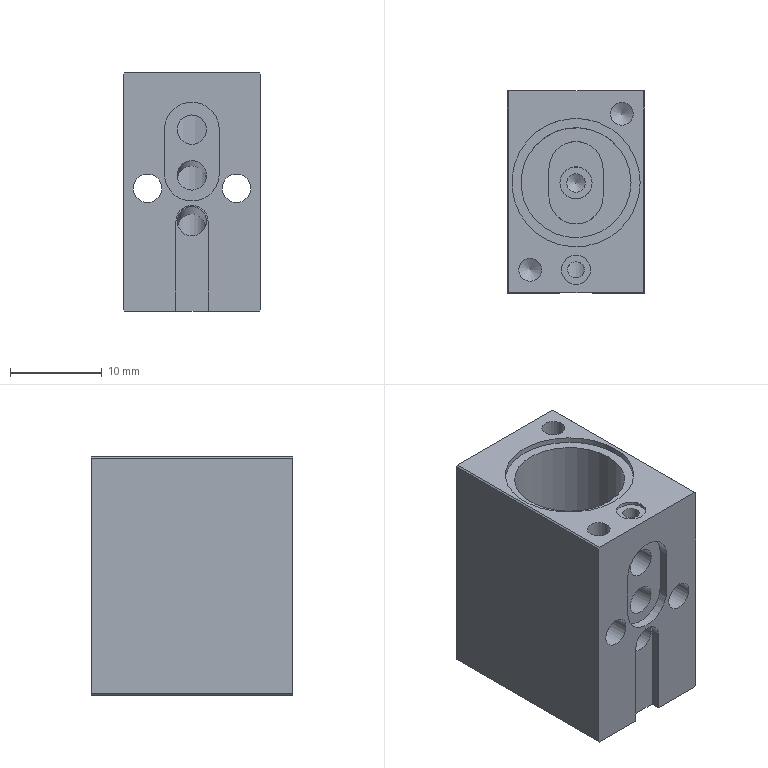NC program | NX | posted with a generic post | part box 15 x 22 x 26 mm
Whole program:
N10 G17 G21 G94 G90
(PLANAR_MILL_2_COPY , TOOL : D3精光)
N12 T05 M6
N14 G54
N16 G17 G0 G90 X-0.215 Y6.8 B0. C0. S3000 M3
N18 G43 Z30. H5
N20 Z1.02
N22 G94 G1 Z-0.98 F300.
N24 Y5.3
N26 G3 X1.285 Y6.8 R1.5
N28 X-0.015 Y8.1 R1.3
N30 X-1.315 Y6.8 R1.3
N32 G1 Y2.
N34 G3 X-0.015 Y0.7 R1.3
N36 X1.285 Y2. R1.3
N38 G1 Y6.8
N40 G3 X0.535 Y7.55 R0.75
N42 G1 Y6.8
N44 Z1.02
N46 G0 Z30.
(PLANAR_MILL_2_COPY_COPY , TOOL : D3精光)
N48 X-0.015
N50 Z1.02
N52 G1 Z-0.98
N54 Y5.3
N56 G3 X1.485 Y6.8 R1.5
N58 X-0.015 Y8.3 R1.5
N60 X-1.515 Y6.8 R1.5
N62 G1 Y2.
N64 G3 X-0.015 Y0.5 R1.5
N66 X1.485 Y2. R1.5
N68 G1 Y6.8
N70 G3 X-0.015 Y8.3 R1.5
N72 G1 Y6.8
N74 Z1.02
N76 G0 Z30.
(PLANAR_MILL_3_COPY , TOOL : D3精光)
N78 X0.25 Y-16.5
N80 Z1.
N82 G1 Z-1.
N84 Y-13.
N86 Y-3.2
N88 G3 X0. Y-2.95 R0.25
N90 X-0.25 Y-3.2 R0.25
N92 G1 Y-13.
N94 Y-16.5
N96 Z1.
N98 G0 Z30.
N100 M5
(PLANAR_MILL_4 , TOOL : D3点钻)
N102 T06 M6
N104 G54
N106 G17 G0 G90 X-9.05 Y0. B0. C0. S4000 M3
N108 G43 Z30. H6
N110 Z1.4
N112 G94 G1 Z-0.6 F1000.
N114 X-8.05
N116 Y12.829
N118 G2 X-7.874 Y13.254 R0.6
N120 G1 X-7.754 Y13.374
N122 G2 X-7.329 Y13.55 R0.6
N124 G1 X7.329
N126 G2 X7.754 Y13.374 R0.6
N128 G1 X7.874 Y13.254
N130 G2 X8.05 Y12.829 R0.6
N132 G1 Y-12.829
N134 G2 X7.874 Y-13.254 R0.6
N136 G1 X7.754 Y-13.374
N138 G2 X7.329 Y-13.55 R0.6
N140 G1 X1.8
N142 G2 X1.2 Y-12.95 R0.6
N144 G1 Y-3.2
N146 G3 X0. Y-2. R1.2
N148 X-1.2 Y-3.2 R1.2
N150 G1 Y-12.95
N152 G2 X-1.8 Y-13.55 R0.6
N154 G1 X-7.329
N156 G2 X-7.754 Y-13.374 R0.6
N158 G1 X-7.874 Y-13.254
N160 G2 X-8.05 Y-12.829 R0.6
N162 G1 Y0.
N164 X-9.05
N166 Z1.4
N168 G0 Z30.
(PLANAR_MILL_5 , TOOL : D3点钻)
N170 X-1.465 Y5.4
N172 Z1.4
N174 G1 Z-0.6
N176 G3 X-2.465 Y4.4 R1.
N178 G1 Y2.
N180 G3 X-0.015 Y-0.45 R2.45
N182 X2.435 Y2. R2.45
N184 G1 Y6.8
N186 G3 X-0.015 Y9.25 R2.45
N188 X-2.465 Y6.8 R2.45
N190 G1 Y4.4
N192 G3 X-1.465 Y3.4 R1.
N194 G1 Z1.4
N196 G0 Z30.
N198 M5
N200 M2